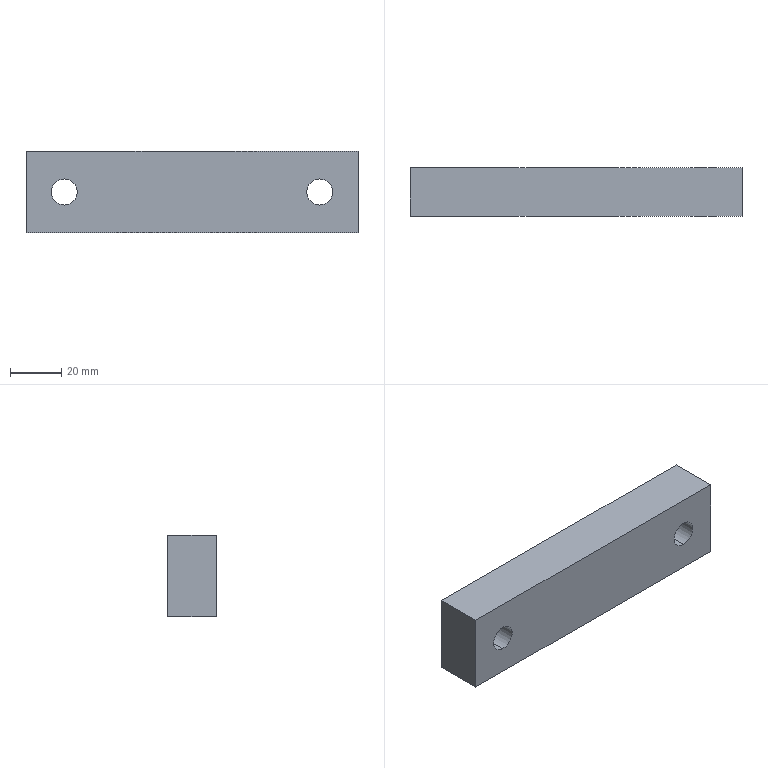Part | SolidWorks | features FlatPattern 1, HoleWzd 1, SMBaseFlange 1, SheetMetal 1 | 1 solid | 10 faces | box 130 x 19 x 32 mm | volume 75935 mm3 | plane 6 | cylinder 4 | commonest cylinder face diameters 10.2 x4
STEP:
#1=CARTESIAN_POINT('',(-50.,-19.,-5.1));
#2=VERTEX_POINT('',#1);
#3=CARTESIAN_POINT('',(-50.,-19.,5.1));
#4=VERTEX_POINT('',#3);
#5=CARTESIAN_POINT('',(-50.,-19.,0.));
#6=DIRECTION('',(0.,1.,0.));
#7=DIRECTION('',(0.,0.,1.));
#8=AXIS2_PLACEMENT_3D('',#5,#6,#7);
#9=CIRCLE('',#8,5.1);
#10=EDGE_CURVE('',#2,#4,#9,.T.);
#11=ORIENTED_EDGE('',*,*,#10,.F.);
#12=CARTESIAN_POINT('',(-50.,0.,-5.1));
#13=VERTEX_POINT('',#12);
#14=CARTESIAN_POINT('',(-50.,0.,-5.1));
#15=DIRECTION('',(0.,1.,0.));
#16=VECTOR('',#15,1000.);
#17=LINE('',#14,#16);
#18=EDGE_CURVE('',#2,#13,#17,.T.);
#19=ORIENTED_EDGE('',*,*,#18,.T.);
#20=CARTESIAN_POINT('',(-50.,0.,5.1));
#21=VERTEX_POINT('',#20);
#22=CARTESIAN_POINT('',(-50.,0.,0.));
#23=DIRECTION('',(0.,1.,0.));
#24=DIRECTION('',(0.,0.,1.));
#25=AXIS2_PLACEMENT_3D('',#22,#23,#24);
#26=CIRCLE('',#25,5.1);
#27=EDGE_CURVE('',#13,#21,#26,.T.);
#28=ORIENTED_EDGE('',*,*,#27,.T.);
#29=CARTESIAN_POINT('',(-50.,0.,5.1));
#30=DIRECTION('',(0.,1.,0.));
#31=VECTOR('',#30,1000.);
#32=LINE('',#29,#31);
#33=EDGE_CURVE('',#4,#21,#32,.T.);
#34=ORIENTED_EDGE('',*,*,#33,.F.);
#35=EDGE_LOOP('',(#11,#19,#28,#34));
#36=FACE_OUTER_BOUND('',#35,.T.);
#37=CARTESIAN_POINT('',(-50.,0.,0.));
#38=DIRECTION('',(0.,1.,0.));
#39=DIRECTION('',(0.,0.,1.));
#40=AXIS2_PLACEMENT_3D('',#37,#38,#39);
#41=CYLINDRICAL_SURFACE('',#40,5.1);
#42=ADVANCED_FACE('',(#36),#41,.F.);
#43=CARTESIAN_POINT('',(50.,-19.,-5.1));
#44=VERTEX_POINT('',#43);
#45=CARTESIAN_POINT('',(50.,-19.,5.1));
#46=VERTEX_POINT('',#45);
#47=CARTESIAN_POINT('',(50.,-19.,0.));
#48=DIRECTION('',(0.,1.,0.));
#49=DIRECTION('',(0.,0.,1.));
#50=AXIS2_PLACEMENT_3D('',#47,#48,#49);
#51=CIRCLE('',#50,5.1);
#52=EDGE_CURVE('',#44,#46,#51,.T.);
#53=ORIENTED_EDGE('',*,*,#52,.F.);
#54=CARTESIAN_POINT('',(50.,0.,-5.1));
#55=VERTEX_POINT('',#54);
#56=CARTESIAN_POINT('',(50.,0.,-5.1));
#57=DIRECTION('',(0.,1.,0.));
#58=VECTOR('',#57,1000.);
#59=LINE('',#56,#58);
#60=EDGE_CURVE('',#44,#55,#59,.T.);
#61=ORIENTED_EDGE('',*,*,#60,.T.);
#62=CARTESIAN_POINT('',(50.,0.,5.1));
#63=VERTEX_POINT('',#62);
#64=CARTESIAN_POINT('',(50.,0.,0.));
#65=DIRECTION('',(0.,1.,0.));
#66=DIRECTION('',(0.,0.,1.));
#67=AXIS2_PLACEMENT_3D('',#64,#65,#66);
#68=CIRCLE('',#67,5.1);
#69=EDGE_CURVE('',#55,#63,#68,.T.);
#70=ORIENTED_EDGE('',*,*,#69,.T.);
#71=CARTESIAN_POINT('',(50.,0.,5.1));
#72=DIRECTION('',(0.,1.,0.));
#73=VECTOR('',#72,1000.);
#74=LINE('',#71,#73);
#75=EDGE_CURVE('',#46,#63,#74,.T.);
#76=ORIENTED_EDGE('',*,*,#75,.F.);
#77=EDGE_LOOP('',(#53,#61,#70,#76));
#78=FACE_OUTER_BOUND('',#77,.T.);
#79=CARTESIAN_POINT('',(50.,0.,0.));
#80=DIRECTION('',(0.,1.,0.));
#81=DIRECTION('',(0.,0.,1.));
#82=AXIS2_PLACEMENT_3D('',#79,#80,#81);
#83=CYLINDRICAL_SURFACE('',#82,5.1);
#84=ADVANCED_FACE('',(#78),#83,.F.);
#85=CARTESIAN_POINT('',(65.,0.,16.));
#86=VERTEX_POINT('',#85);
#87=CARTESIAN_POINT('',(65.,0.,-16.));
#88=VERTEX_POINT('',#87);
#89=CARTESIAN_POINT('',(65.,0.,-16.));
#90=DIRECTION('',(0.,0.,-1.));
#91=VECTOR('',#90,1000.);
#92=LINE('',#89,#91);
#93=EDGE_CURVE('',#86,#88,#92,.T.);
#94=ORIENTED_EDGE('',*,*,#93,.F.);
#95=CARTESIAN_POINT('',(65.,-19.,16.));
#96=VERTEX_POINT('',#95);
#97=CARTESIAN_POINT('',(65.,-19.,16.));
#98=DIRECTION('',(0.,1.,0.));
#99=VECTOR('',#98,1000.);
#100=LINE('',#97,#99);
#101=EDGE_CURVE('',#96,#86,#100,.T.);
#102=ORIENTED_EDGE('',*,*,#101,.F.);
#103=CARTESIAN_POINT('',(65.,-19.,-16.));
#104=VERTEX_POINT('',#103);
#105=CARTESIAN_POINT('',(65.,-19.,-16.));
#106=DIRECTION('',(0.,0.,-1.));
#107=VECTOR('',#106,1000.);
#108=LINE('',#105,#107);
#109=EDGE_CURVE('',#96,#104,#108,.T.);
#110=ORIENTED_EDGE('',*,*,#109,.T.);
#111=CARTESIAN_POINT('',(65.,-19.,-16.));
#112=DIRECTION('',(0.,1.,0.));
#113=VECTOR('',#112,1000.);
#114=LINE('',#111,#113);
#115=EDGE_CURVE('',#104,#88,#114,.T.);
#116=ORIENTED_EDGE('',*,*,#115,.T.);
#117=EDGE_LOOP('',(#94,#102,#110,#116));
#118=FACE_OUTER_BOUND('',#117,.T.);
#119=CARTESIAN_POINT('',(65.,-19.,-16.));
#120=DIRECTION('',(1.,0.,0.));
#121=DIRECTION('',(0.,0.,-1.));
#122=AXIS2_PLACEMENT_3D('',#119,#120,#121);
#123=PLANE('',#122);
#124=ADVANCED_FACE('',(#118),#123,.T.);
#125=CARTESIAN_POINT('',(-65.,0.,16.));
#126=VERTEX_POINT('',#125);
#127=CARTESIAN_POINT('',(-65.,0.,16.));
#128=DIRECTION('',(1.,0.,0.));
#129=VECTOR('',#128,1000.);
#130=LINE('',#127,#129);
#131=EDGE_CURVE('',#126,#86,#130,.T.);
#132=ORIENTED_EDGE('',*,*,#131,.F.);
#133=CARTESIAN_POINT('',(-65.,-19.,16.));
#134=VERTEX_POINT('',#133);
#135=CARTESIAN_POINT('',(-65.,-19.,16.));
#136=DIRECTION('',(0.,1.,0.));
#137=VECTOR('',#136,1000.);
#138=LINE('',#135,#137);
#139=EDGE_CURVE('',#134,#126,#138,.T.);
#140=ORIENTED_EDGE('',*,*,#139,.F.);
#141=CARTESIAN_POINT('',(-65.,-19.,16.));
#142=DIRECTION('',(1.,0.,0.));
#143=VECTOR('',#142,1000.);
#144=LINE('',#141,#143);
#145=EDGE_CURVE('',#134,#96,#144,.T.);
#146=ORIENTED_EDGE('',*,*,#145,.T.);
#147=ORIENTED_EDGE('',*,*,#101,.T.);
#148=EDGE_LOOP('',(#132,#140,#146,#147));
#149=FACE_OUTER_BOUND('',#148,.T.);
#150=CARTESIAN_POINT('',(-65.,-19.,16.));
#151=DIRECTION('',(0.,0.,1.));
#152=DIRECTION('',(1.,0.,0.));
#153=AXIS2_PLACEMENT_3D('',#150,#151,#152);
#154=PLANE('',#153);
#155=ADVANCED_FACE('',(#149),#154,.T.);
#156=CARTESIAN_POINT('',(-65.,0.,-16.));
#157=VERTEX_POINT('',#156);
#158=CARTESIAN_POINT('',(-65.,0.,-16.));
#159=DIRECTION('',(0.,0.,1.));
#160=VECTOR('',#159,1000.);
#161=LINE('',#158,#160);
#162=EDGE_CURVE('',#157,#126,#161,.T.);
#163=ORIENTED_EDGE('',*,*,#162,.F.);
#164=CARTESIAN_POINT('',(-65.,-19.,-16.));
#165=VERTEX_POINT('',#164);
#166=CARTESIAN_POINT('',(-65.,-19.,-16.));
#167=DIRECTION('',(0.,1.,0.));
#168=VECTOR('',#167,1000.);
#169=LINE('',#166,#168);
#170=EDGE_CURVE('',#165,#157,#169,.T.);
#171=ORIENTED_EDGE('',*,*,#170,.F.);
#172=CARTESIAN_POINT('',(-65.,-19.,-16.));
#173=DIRECTION('',(0.,0.,1.));
#174=VECTOR('',#173,1000.);
#175=LINE('',#172,#174);
#176=EDGE_CURVE('',#165,#134,#175,.T.);
#177=ORIENTED_EDGE('',*,*,#176,.T.);
#178=ORIENTED_EDGE('',*,*,#139,.T.);
#179=EDGE_LOOP('',(#163,#171,#177,#178));
#180=FACE_OUTER_BOUND('',#179,.T.);
#181=CARTESIAN_POINT('',(-65.,-19.,-16.));
#182=DIRECTION('',(-1.,0.,0.));
#183=DIRECTION('',(0.,0.,1.));
#184=AXIS2_PLACEMENT_3D('',#181,#182,#183);
#185=PLANE('',#184);
#186=ADVANCED_FACE('',(#180),#185,.T.);
#187=CARTESIAN_POINT('',(-65.,0.,-16.));
#188=DIRECTION('',(-1.,0.,0.));
#189=VECTOR('',#188,1000.);
#190=LINE('',#187,#189);
#191=EDGE_CURVE('',#88,#157,#190,.T.);
#192=ORIENTED_EDGE('',*,*,#191,.F.);
#193=ORIENTED_EDGE('',*,*,#115,.F.);
#194=CARTESIAN_POINT('',(-65.,-19.,-16.));
#195=DIRECTION('',(-1.,0.,0.));
#196=VECTOR('',#195,1000.);
#197=LINE('',#194,#196);
#198=EDGE_CURVE('',#104,#165,#197,.T.);
#199=ORIENTED_EDGE('',*,*,#198,.T.);
#200=ORIENTED_EDGE('',*,*,#170,.T.);
#201=EDGE_LOOP('',(#192,#193,#199,#200));
#202=FACE_OUTER_BOUND('',#201,.T.);
#203=CARTESIAN_POINT('',(-65.,-19.,-16.));
#204=DIRECTION('',(0.,0.,-1.));
#205=DIRECTION('',(-1.,0.,0.));
#206=AXIS2_PLACEMENT_3D('',#203,#204,#205);
#207=PLANE('',#206);
#208=ADVANCED_FACE('',(#202),#207,.T.);
#209=CARTESIAN_POINT('',(-50.,-19.,0.));
#210=DIRECTION('',(0.,1.,0.));
#211=DIRECTION('',(0.,0.,1.));
#212=AXIS2_PLACEMENT_3D('',#209,#210,#211);
#213=CIRCLE('',#212,5.1);
#214=EDGE_CURVE('',#4,#2,#213,.T.);
#215=ORIENTED_EDGE('',*,*,#214,.T.);
#216=ORIENTED_EDGE('',*,*,#10,.T.);
#217=EDGE_LOOP('',(#215,#216));
#218=FACE_BOUND('',#217,.T.);
#219=CARTESIAN_POINT('',(50.,-19.,0.));
#220=DIRECTION('',(0.,1.,0.));
#221=DIRECTION('',(0.,0.,1.));
#222=AXIS2_PLACEMENT_3D('',#219,#220,#221);
#223=CIRCLE('',#222,5.1);
#224=EDGE_CURVE('',#46,#44,#223,.T.);
#225=ORIENTED_EDGE('',*,*,#224,.T.);
#226=ORIENTED_EDGE('',*,*,#52,.T.);
#227=EDGE_LOOP('',(#225,#226));
#228=FACE_BOUND('',#227,.T.);
#229=ORIENTED_EDGE('',*,*,#109,.F.);
#230=ORIENTED_EDGE('',*,*,#145,.F.);
#231=ORIENTED_EDGE('',*,*,#176,.F.);
#232=ORIENTED_EDGE('',*,*,#198,.F.);
#233=EDGE_LOOP('',(#229,#230,#231,#232));
#234=FACE_OUTER_BOUND('',#233,.T.);
#235=CARTESIAN_POINT('',(0.,-19.,0.));
#236=DIRECTION('',(0.,1.,0.));
#237=DIRECTION('',(0.,0.,1.));
#238=AXIS2_PLACEMENT_3D('',#235,#236,#237);
#239=PLANE('',#238);
#240=ADVANCED_FACE('',(#218,#228,#234),#239,.F.);
#241=CARTESIAN_POINT('',(-50.,0.,0.));
#242=DIRECTION('',(0.,1.,0.));
#243=DIRECTION('',(0.,0.,1.));
#244=AXIS2_PLACEMENT_3D('',#241,#242,#243);
#245=CIRCLE('',#244,5.1);
#246=EDGE_CURVE('',#21,#13,#245,.T.);
#247=ORIENTED_EDGE('',*,*,#246,.F.);
#248=ORIENTED_EDGE('',*,*,#27,.F.);
#249=EDGE_LOOP('',(#247,#248));
#250=FACE_BOUND('',#249,.T.);
#251=CARTESIAN_POINT('',(50.,0.,0.));
#252=DIRECTION('',(0.,1.,0.));
#253=DIRECTION('',(0.,0.,1.));
#254=AXIS2_PLACEMENT_3D('',#251,#252,#253);
#255=CIRCLE('',#254,5.1);
#256=EDGE_CURVE('',#63,#55,#255,.T.);
#257=ORIENTED_EDGE('',*,*,#256,.F.);
#258=ORIENTED_EDGE('',*,*,#69,.F.);
#259=EDGE_LOOP('',(#257,#258));
#260=FACE_BOUND('',#259,.T.);
#261=ORIENTED_EDGE('',*,*,#93,.T.);
#262=ORIENTED_EDGE('',*,*,#191,.T.);
#263=ORIENTED_EDGE('',*,*,#162,.T.);
#264=ORIENTED_EDGE('',*,*,#131,.T.);
#265=EDGE_LOOP('',(#261,#262,#263,#264));
#266=FACE_OUTER_BOUND('',#265,.T.);
#267=CARTESIAN_POINT('',(0.,0.,0.));
#268=DIRECTION('',(0.,1.,0.));
#269=DIRECTION('',(0.,0.,1.));
#270=AXIS2_PLACEMENT_3D('',#267,#268,#269);
#271=PLANE('',#270);
#272=ADVANCED_FACE('',(#250,#260,#266),#271,.T.);
#273=ORIENTED_EDGE('',*,*,#60,.F.);
#274=ORIENTED_EDGE('',*,*,#224,.F.);
#275=ORIENTED_EDGE('',*,*,#75,.T.);
#276=ORIENTED_EDGE('',*,*,#256,.T.);
#277=EDGE_LOOP('',(#273,#274,#275,#276));
#278=FACE_OUTER_BOUND('',#277,.T.);
#279=CARTESIAN_POINT('',(50.,0.,0.));
#280=DIRECTION('',(0.,1.,0.));
#281=DIRECTION('',(0.,0.,1.));
#282=AXIS2_PLACEMENT_3D('',#279,#280,#281);
#283=CYLINDRICAL_SURFACE('',#282,5.1);
#284=ADVANCED_FACE('',(#278),#283,.F.);
#285=ORIENTED_EDGE('',*,*,#18,.F.);
#286=ORIENTED_EDGE('',*,*,#214,.F.);
#287=ORIENTED_EDGE('',*,*,#33,.T.);
#288=ORIENTED_EDGE('',*,*,#246,.T.);
#289=EDGE_LOOP('',(#285,#286,#287,#288));
#290=FACE_OUTER_BOUND('',#289,.T.);
#291=CARTESIAN_POINT('',(-50.,0.,0.));
#292=DIRECTION('',(0.,1.,0.));
#293=DIRECTION('',(0.,0.,1.));
#294=AXIS2_PLACEMENT_3D('',#291,#292,#293);
#295=CYLINDRICAL_SURFACE('',#294,5.1);
#296=ADVANCED_FACE('',(#290),#295,.F.);
#297=CLOSED_SHELL('',(#42,#84,#124,#155,#186,#208,#240,#272,#284,#296));
#298=MANIFOLD_SOLID_BREP('',#297);
#299=CARTESIAN_POINT('',(0.,0.,0.));
#300=DIRECTION('',(0.,0.,1.));
#301=DIRECTION('',(1.,0.,0.));
#302=AXIS2_PLACEMENT_3D('',#299,#300,#301);
#303=(LENGTH_UNIT()NAMED_UNIT(*)SI_UNIT(.MILLI.,.METRE.));
#304=UNCERTAINTY_MEASURE_WITH_UNIT(LENGTH_MEASURE(0.00001),#303,'','');
#305=(NAMED_UNIT(*)PLANE_ANGLE_UNIT()SI_UNIT($,.RADIAN.));
#306=(NAMED_UNIT(*)SI_UNIT($,.STERADIAN.)SOLID_ANGLE_UNIT());
#307=(GEOMETRIC_REPRESENTATION_CONTEXT(3)GLOBAL_UNCERTAINTY_ASSIGNED_CONTEXT((#304))GLOBAL_UNIT_ASSIGNED_CONTEXT((#303,#305,#306))REPRESENTATION_CONTEXT('',''));
#308=ADVANCED_BREP_SHAPE_REPRESENTATION('',(#298,#302),#307);